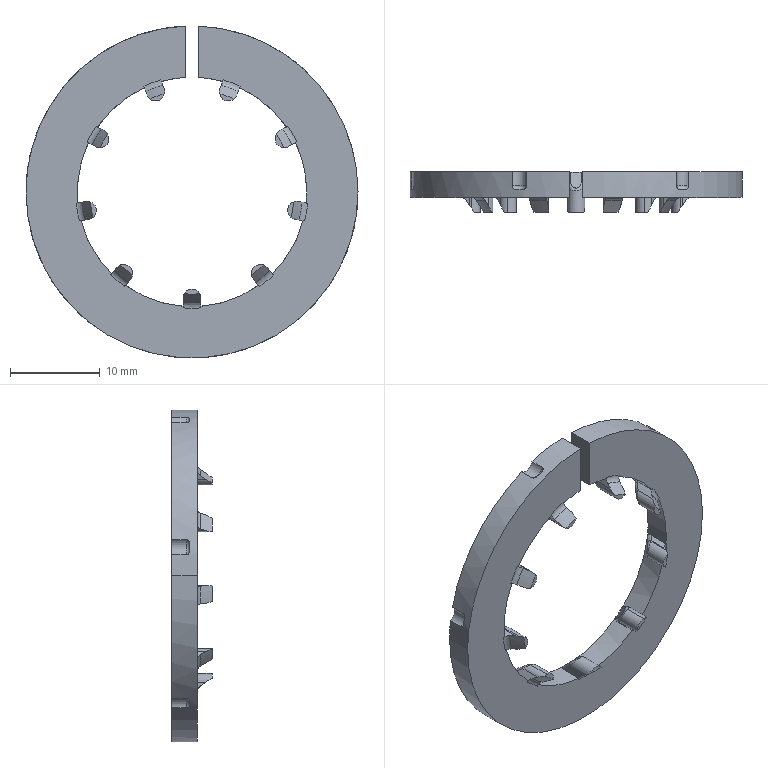Part | SolidWorks | features BaseBody 1 | 1 solid | 134 faces | box 36.9 x 4.5 x 36.885 mm | volume 1647 mm3 | plane 37 | cylinder 35 | spline 28 | cone 18 | torus 16 | commonest cylinder face diameters 2 x21 25.5 x11 36.9 x3